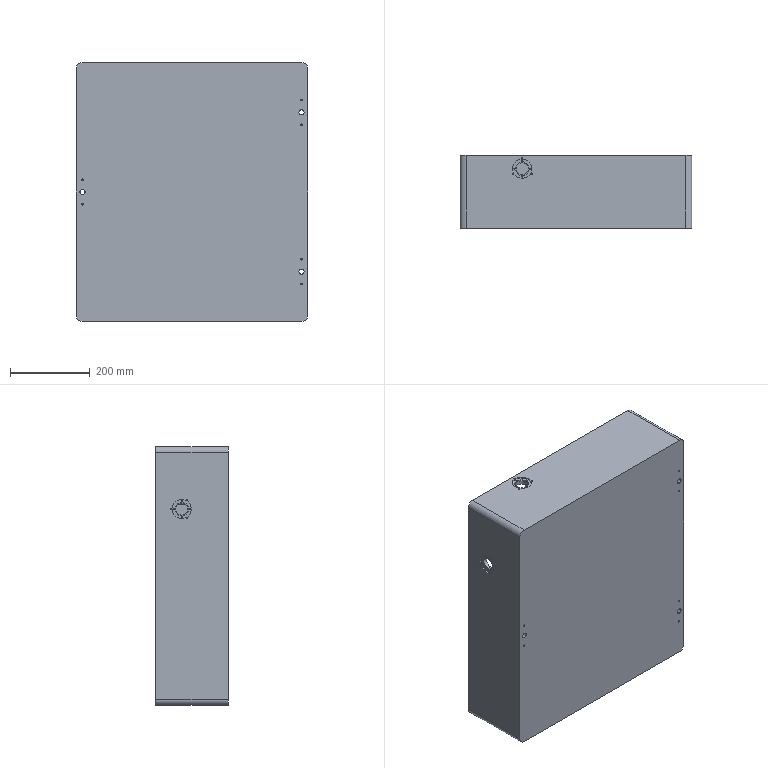Part | SolidWorks | features ICE 20, HoleWzd 13, Fillet 6, Chamfer 1, Extrusion 1, Shell 1 | 1 solid | 1478 faces | box 582 x 183 x 650 mm | volume 11923446 mm3 | cylinder 983 | cone 396 | plane 99 | commonest cylinder face diameters 2.5 x746 3.3 x134 10 x27 5 x8 20 x8 30 x8